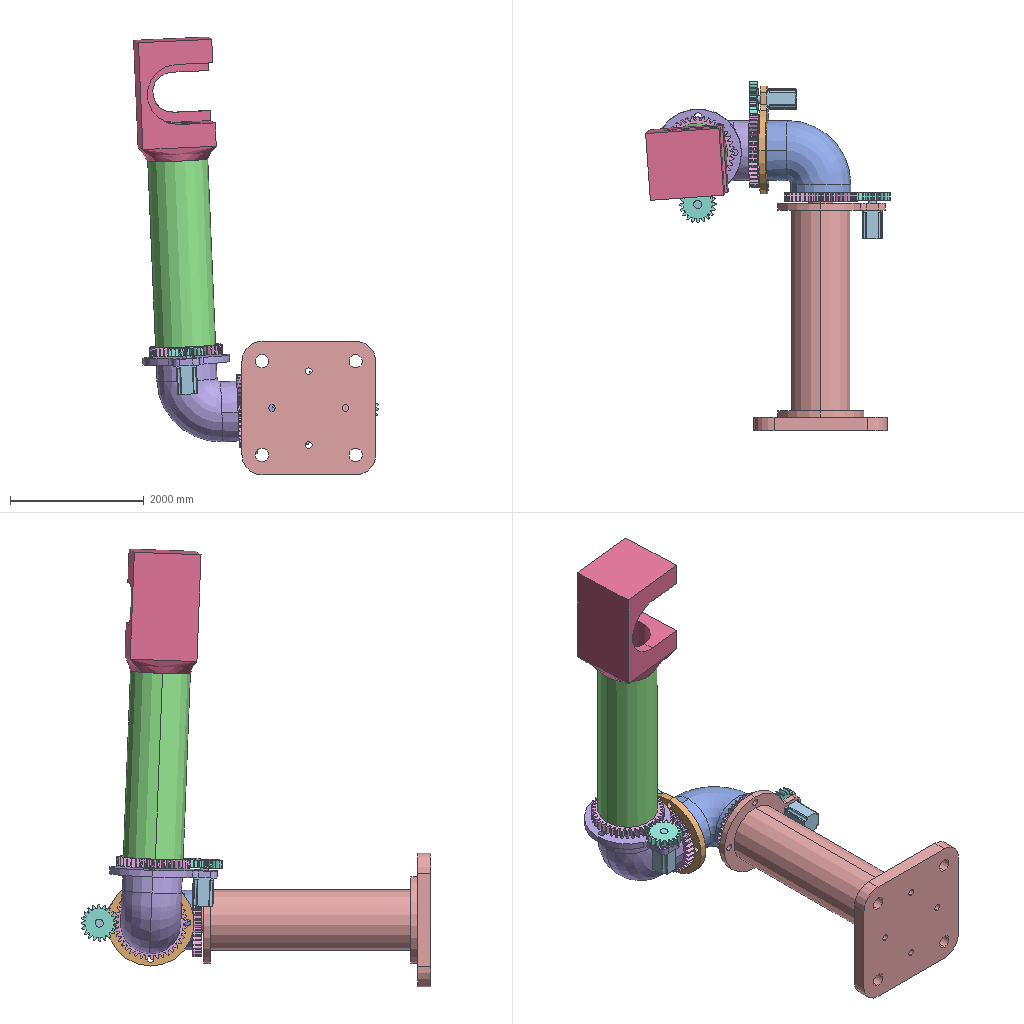Assembly | SolidWorks | 10 different items | 18 placed | box 3661 x 5231 x 6547 mm
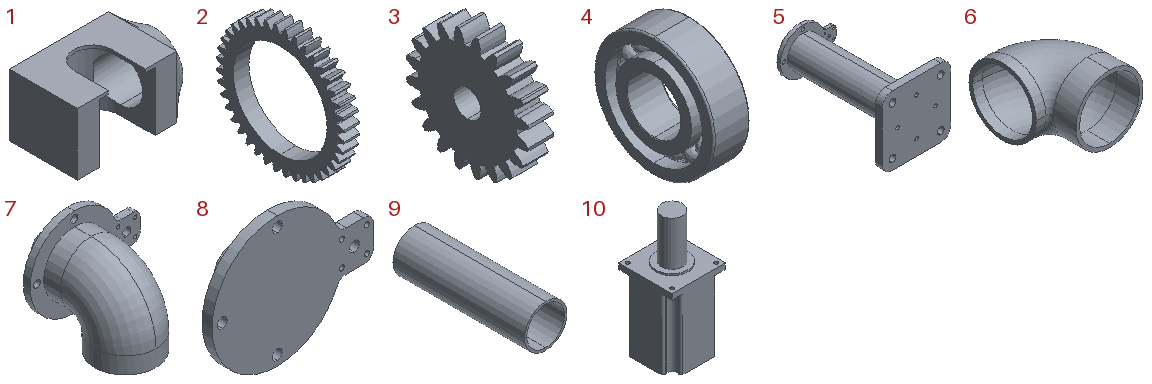Parts list (item | quantity | size | volume | features):
1 | x1 | 1800 x 1100 x 1000 mm | 917422544 mm3 | features ICE 3, Blend 1, Extrusion 1
2 | x3 | 132.6 x 1090 x 1090 mm | 44239746 mm3 | features ICE 2, BaseBody 1, Scale 1
3 | x3 | 112.2 x 539.706 x 539.706 mm | 19588438 mm3 | features ICE 2, BaseBody 1, Scale 1
4 | x3 | 240 x 800 x 800 mm | 68366602 mm3 | features BaseBody 1, Scale 1
5 | x1 | 2000 x 3750 x 2000 mm | 2968644378 mm3 | features ICE 8, Extrusion 1, Fillet 1, MirrorPattern 1
6 | x1 | 1080 x 1250 x 900 mm | 162277153 mm3 | features ICE 3, MoveFace 3, Extrusion 1, Sweep 1
7 | x1 | 1613 x 1648 x 1392 mm | 988148338 mm3 | features ICE 9, MoveFace 2, Extrusion 1, Fillet 1, MirrorPattern 1, Sweep 1
8 | x1 | 1613 x 450 x 1300 mm | 177120660 mm3 | features ICE 9, Extrusion 1, Fillet 1, MirrorPattern 1
9 | x1 | 900 x 2782 x 900 mm | 371446207 mm3 | features Extrusion 1, MoveFace 1
10 | x3 | 300 x 300 x 687.5 mm | 37123455 mm3 | features BaseBody 1, ICE 1, Scale 1
Mates (type | each side: item.copy, entity, surface, feature):
Concentric | 5.1 face cylinder Boss-Extrude5 | 4.1 face cylinder Input1
Coincident | 4.1 face plane Input1 | 2.1 face plane Boss-Extrude1
Concentric | 5.1 face cylinder Boss-Extrude1 | 6.1 face cylinder Sweep1
Concentric | 4.1 face cylinder Input1 | 2.1 face cylinder Cut-Extrude1
Parallel | 4.1 face plane Input1 | 2.1 face plane Input1
Coincident | 6.1 face plane Sweep1 | 2.1 face plane Input1
Parallel | 6.1 select_type:24 | 2.1 select_type:24
Coincident | 2.1 face plane Input1 | 3.1 face plane Boss-Extrude1
Concentric | 6.1 face cylinder Boss-Extrude1 | 8.1 face cylinder Mirror1
Coincident | 6.1 face plane Cut-Extrude2 | 8.1 face plane Mirror1
Parallel | 2.1 select_type:24 | 8.1 edge
Concentric | 4.2 face cylinder Input1 | 8.1 face cylinder Boss-Extrude5
Coincident | 4.2 face plane Input1 | 8.1 face plane Boss-Extrude5
Coincident | 3.2 face plane Boss-Extrude1 | 2.2 face plane Boss-Extrude1
Concentric | 6.1 face cylinder Boss-Extrude1 | 7.1 face cylinder Sweep1
Concentric | 4.2 face cylinder Input1 | 7.1 face cylinder Sweep1
Coincident | 2.2 face plane Boss-Extrude1 | 7.1 face plane Sweep1
Parallel | 2.2 select_type:24 | 7.1 select_type:24
Concentric | 2.2 face cylinder Cut-Extrude1 | 7.1 face cylinder Sweep1
Concentric | 7.1 face cylinder Boss-Extrude5 | 4.3 face cylinder Input1
Coincident | 7.1 face plane Boss-Extrude5 | 4.3 face plane Input1
Concentric | 4.3 face cylinder Input1 | 2.3 face cylinder Cut-Extrude1
Coincident | 3.3 face plane Boss-Extrude1 | 2.3 face plane Boss-Extrude1
Coincident | 2.3 face plane Boss-Extrude1 | 9.1 face plane Boss-Extrude1
Concentric | 4.3 face cylinder Input1 | 9.1 face cylinder Boss-Extrude1
Parallel | 2.3 select_type:24 | 9.1 select_type:24
Coincident | 9.1 face plane Boss-Extrude1 | 1.1 face plane Loft1
Coincident | 9.1 face cylinder Boss-Extrude1 | 1.1 edge
Parallel | 2.3 select_type:24 | 1.1 face plane Boss-Extrude1
Coincident | 5.1 face plane Mirror1 | 10.1 face plane Input1
Concentric | 5.1 face cylinder Cut-Extrude3 | 10.1 face cylinder Input1
Concentric | 3.1 face cylinder Cut-Extrude1 | 10.1 face cylinder Boss-Extrude1
Coincident | 3.1 face plane Boss-Extrude1 | 10.1 face plane Boss-Extrude1
Concentric | 5.1 face cylinder Cut-Extrude3 | 10.1 face cylinder Boss-Extrude1
Concentric | 8.1 face cylinder Cut-Extrude3 | 10.2 face cylinder Boss-Extrude1
Coincident | 8.1 face plane Mirror1 | 10.2 face plane Input1
Concentric | 3.2 face cylinder Cut-Extrude1 | 10.2 face cylinder Boss-Extrude1
Coincident | 3.2 face plane Boss-Extrude1 | 10.2 face plane Boss-Extrude1
Concentric | 7.1 face cylinder Cut-Extrude3 | 10.3 face cylinder Boss-Extrude1
Coincident | 7.1 face plane Mirror1 | 10.3 face plane Input1
Concentric | 7.1 face cylinder Cut-Extrude3 | 10.3 face cylinder Input1 | 2 times
Concentric | 3.3 face cylinder Cut-Extrude1 | 10.3 face cylinder Boss-Extrude1
Coincident | 3.3 face plane Boss-Extrude1 | 10.3 face plane Boss-Extrude1